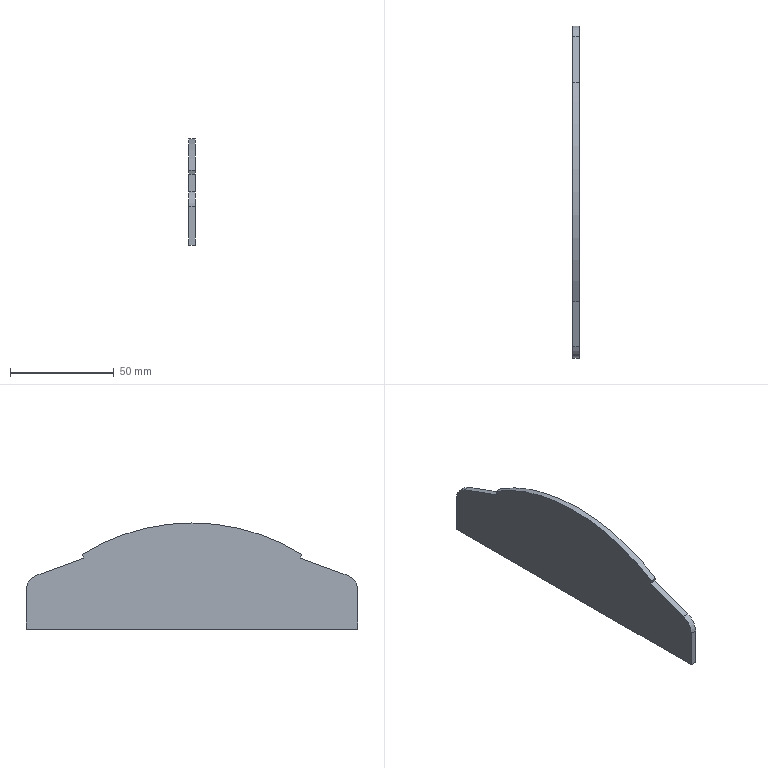Part | STEP file | 1-43.9 | 1 solid | 12 faces | box 3 x 160 x 51.122 mm | volume 19342 mm3 | plane 9 | cylinder 3 | commonest cylinder face diameters 16 x2 200 x1
STEP:
#1=CARTESIAN_POINT('',(0.,0.,0.));
#2=DIRECTION('',(0.,0.,1.));
#3=DIRECTION('',(1.,0.,0.));
#4=AXIS2_PLACEMENT_3D('',#1,#2,#3);
#5=CARTESIAN_POINT('',(0.,-80.,-12.));
#6=VERTEX_POINT('',#5);
#7=CARTESIAN_POINT('',(0.,80.,-12.));
#8=VERTEX_POINT('',#7);
#9=CARTESIAN_POINT('',(0.,-80.,-12.));
#10=DIRECTION('',(0.,1.,0.));
#11=VECTOR('',#10,1.);
#12=LINE('',#9,#11);
#13=CARTESIAN_POINT('',(0.,0.,68.));
#14=DIRECTION('',(1.,0.,0.));
#15=DIRECTION('',(0.,1.,0.));
#16=AXIS2_PLACEMENT_3D('',#13,#14,#15);
#17=PLANE('',#16);
#18=CARTESIAN_POINT('',(-80.,-80.));
#19=DIRECTION('',(1.,0.));
#20=VECTOR('',#19,1.);
#21=LINE('',#18,#20);
#22=(GEOMETRIC_REPRESENTATION_CONTEXT(2)PARAMETRIC_REPRESENTATION_CONTEXT()REPRESENTATION_CONTEXT('',''));
#23=DEFINITIONAL_REPRESENTATION('',(#21),#22);
#24=PCURVE('',#17,#23);
#25=CARTESIAN_POINT('',(-1.5,0.,-12.));
#26=DIRECTION('',(0.,0.,1.));
#27=DIRECTION('',(0.,1.,0.));
#28=AXIS2_PLACEMENT_3D('',#25,#26,#27);
#29=PLANE('',#28);
#30=CARTESIAN_POINT('',(-80.,-1.5));
#31=DIRECTION('',(1.,0.));
#32=VECTOR('',#31,1.);
#33=LINE('',#30,#32);
#34=(GEOMETRIC_REPRESENTATION_CONTEXT(2)PARAMETRIC_REPRESENTATION_CONTEXT()REPRESENTATION_CONTEXT('',''));
#35=DEFINITIONAL_REPRESENTATION('',(#33),#34);
#36=PCURVE('',#29,#35);
#37=SURFACE_CURVE('',#12,(#24,#36),.PCURVE_S1.);
#38=EDGE_CURVE('',#6,#8,#37,.T.);
#39=ORIENTED_EDGE('',*,*,#38,.T.);
#40=CARTESIAN_POINT('',(0.,80.,6.398));
#41=VERTEX_POINT('',#40);
#42=CARTESIAN_POINT('',(0.,80.,-12.));
#43=DIRECTION('',(0.,0.,1.));
#44=VECTOR('',#43,1.);
#45=LINE('',#42,#44);
#46=CARTESIAN_POINT('',(80.,-80.));
#47=DIRECTION('',(0.,1.));
#48=VECTOR('',#47,1.);
#49=LINE('',#46,#48);
#50=(GEOMETRIC_REPRESENTATION_CONTEXT(2)PARAMETRIC_REPRESENTATION_CONTEXT()REPRESENTATION_CONTEXT('',''));
#51=DEFINITIONAL_REPRESENTATION('',(#49),#50);
#52=PCURVE('',#17,#51);
#53=CARTESIAN_POINT('',(-1.5,80.,-2.801));
#54=DIRECTION('',(0.,-1.,0.));
#55=DIRECTION('',(0.,0.,1.));
#56=AXIS2_PLACEMENT_3D('',#53,#54,#55);
#57=PLANE('',#56);
#58=CARTESIAN_POINT('',(-9.199,-1.5));
#59=DIRECTION('',(1.,0.));
#60=VECTOR('',#59,1.);
#61=LINE('',#58,#60);
#62=(GEOMETRIC_REPRESENTATION_CONTEXT(2)PARAMETRIC_REPRESENTATION_CONTEXT()REPRESENTATION_CONTEXT('',''));
#63=DEFINITIONAL_REPRESENTATION('',(#61),#62);
#64=PCURVE('',#57,#63);
#65=SURFACE_CURVE('',#45,(#52,#64),.PCURVE_S1.);
#66=EDGE_CURVE('',#8,#41,#65,.T.);
#67=ORIENTED_EDGE('',*,*,#66,.T.);
#68=CARTESIAN_POINT('',(0.,74.736,13.916));
#69=VERTEX_POINT('',#68);
#70=CARTESIAN_POINT('',(0.,72.,6.398));
#71=DIRECTION('',(1.,0.,0.));
#72=DIRECTION('',(0.,1.,0.));
#73=AXIS2_PLACEMENT_3D('',#70,#71,#72);
#74=CIRCLE('',#73,8.);
#75=CARTESIAN_POINT('',(72.,-61.602));
#76=DIRECTION('',(1.,0.));
#77=AXIS2_PLACEMENT_2D('',#75,#76);
#78=CIRCLE('',#77,8.);
#79=(GEOMETRIC_REPRESENTATION_CONTEXT(2)PARAMETRIC_REPRESENTATION_CONTEXT()REPRESENTATION_CONTEXT('',''));
#80=DEFINITIONAL_REPRESENTATION('',(#78),#79);
#81=PCURVE('',#17,#80);
#82=CARTESIAN_POINT('',(0.,72.,6.398));
#83=DIRECTION('',(-1.,0.,0.));
#84=DIRECTION('',(0.,1.,0.));
#85=AXIS2_PLACEMENT_3D('',#82,#83,#84);
#86=CYLINDRICAL_SURFACE('',#85,8.);
#87=CARTESIAN_POINT('',(6.283,0.));
#88=DIRECTION('',(-1.,0.));
#89=VECTOR('',#88,1.);
#90=LINE('',#87,#89);
#91=(GEOMETRIC_REPRESENTATION_CONTEXT(2)PARAMETRIC_REPRESENTATION_CONTEXT()REPRESENTATION_CONTEXT('',''));
#92=DEFINITIONAL_REPRESENTATION('',(#90),#91);
#93=PCURVE('',#86,#92);
#94=SURFACE_CURVE('',#74,(#81,#93),.PCURVE_S1.);
#95=EDGE_CURVE('',#41,#69,#94,.T.);
#96=ORIENTED_EDGE('',*,*,#95,.T.);
#97=CARTESIAN_POINT('',(0.,52.185,22.124));
#98=VERTEX_POINT('',#97);
#99=CARTESIAN_POINT('',(0.,74.736,13.916));
#100=DIRECTION('',(0.,-0.9397,0.342));
#101=VECTOR('',#100,1.);
#102=LINE('',#99,#101);
#103=CARTESIAN_POINT('',(74.736,-54.084));
#104=DIRECTION('',(-0.9397,0.342));
#105=VECTOR('',#104,1.);
#106=LINE('',#103,#105);
#107=(GEOMETRIC_REPRESENTATION_CONTEXT(2)PARAMETRIC_REPRESENTATION_CONTEXT()REPRESENTATION_CONTEXT('',''));
#108=DEFINITIONAL_REPRESENTATION('',(#106),#107);
#109=PCURVE('',#17,#108);
#110=CARTESIAN_POINT('',(-1.5,63.461,18.02));
#111=DIRECTION('',(0.,-0.342,-0.9397));
#112=DIRECTION('',(0.,-0.9397,0.342));
#113=AXIS2_PLACEMENT_3D('',#110,#111,#112);
#114=PLANE('',#113);
#115=CARTESIAN_POINT('',(-11.999,-1.5));
#116=DIRECTION('',(1.,0.));
#117=VECTOR('',#116,1.);
#118=LINE('',#115,#117);
#119=(GEOMETRIC_REPRESENTATION_CONTEXT(2)PARAMETRIC_REPRESENTATION_CONTEXT()REPRESENTATION_CONTEXT('',''));
#120=DEFINITIONAL_REPRESENTATION('',(#118),#119);
#121=PCURVE('',#114,#120);
#122=SURFACE_CURVE('',#102,(#109,#121),.PCURVE_S1.);
#123=EDGE_CURVE('',#69,#98,#122,.T.);
#124=ORIENTED_EDGE('',*,*,#123,.T.);
#125=CARTESIAN_POINT('',(0.,52.869,24.003));
#126=VERTEX_POINT('',#125);
#127=CARTESIAN_POINT('',(0.,52.185,22.124));
#128=DIRECTION('',(0.,0.342,0.9397));
#129=VECTOR('',#128,1.);
#130=LINE('',#127,#129);
#131=CARTESIAN_POINT('',(52.185,-45.876));
#132=DIRECTION('',(0.342,0.9397));
#133=VECTOR('',#132,1.);
#134=LINE('',#131,#133);
#135=(GEOMETRIC_REPRESENTATION_CONTEXT(2)PARAMETRIC_REPRESENTATION_CONTEXT()REPRESENTATION_CONTEXT('',''));
#136=DEFINITIONAL_REPRESENTATION('',(#134),#135);
#137=PCURVE('',#17,#136);
#138=CARTESIAN_POINT('',(-1.5,52.527,23.063));
#139=DIRECTION('',(0.,-0.9397,0.342));
#140=DIRECTION('',(0.,0.342,0.9397));
#141=AXIS2_PLACEMENT_3D('',#138,#139,#140);
#142=PLANE('',#141);
#143=CARTESIAN_POINT('',(-1.,-1.5));
#144=DIRECTION('',(1.,0.));
#145=VECTOR('',#144,1.);
#146=LINE('',#143,#145);
#147=(GEOMETRIC_REPRESENTATION_CONTEXT(2)PARAMETRIC_REPRESENTATION_CONTEXT()REPRESENTATION_CONTEXT('',''));
#148=DEFINITIONAL_REPRESENTATION('',(#146),#147);
#149=PCURVE('',#142,#148);
#150=SURFACE_CURVE('',#130,(#137,#149),.PCURVE_S1.);
#151=EDGE_CURVE('',#98,#126,#150,.T.);
#152=ORIENTED_EDGE('',*,*,#151,.T.);
#153=CARTESIAN_POINT('',(0.,-52.869,24.003));
#154=VERTEX_POINT('',#153);
#155=CARTESIAN_POINT('',(0.,0.,-60.878));
#156=DIRECTION('',(1.,0.,0.));
#157=DIRECTION('',(0.,0.5287,0.8488));
#158=AXIS2_PLACEMENT_3D('',#155,#156,#157);
#159=CIRCLE('',#158,100.);
#160=CARTESIAN_POINT('',(0.,-128.878));
#161=DIRECTION('',(0.5287,0.8488));
#162=AXIS2_PLACEMENT_2D('',#160,#161);
#163=CIRCLE('',#162,100.);
#164=(GEOMETRIC_REPRESENTATION_CONTEXT(2)PARAMETRIC_REPRESENTATION_CONTEXT()REPRESENTATION_CONTEXT('',''));
#165=DEFINITIONAL_REPRESENTATION('',(#163),#164);
#166=PCURVE('',#17,#165);
#167=CARTESIAN_POINT('',(0.,0.,-60.878));
#168=DIRECTION('',(-1.,0.,0.));
#169=DIRECTION('',(0.,0.5287,0.8488));
#170=AXIS2_PLACEMENT_3D('',#167,#168,#169);
#171=CYLINDRICAL_SURFACE('',#170,100.);
#172=CARTESIAN_POINT('',(6.283,0.));
#173=DIRECTION('',(-1.,0.));
#174=VECTOR('',#173,1.);
#175=LINE('',#172,#174);
#176=(GEOMETRIC_REPRESENTATION_CONTEXT(2)PARAMETRIC_REPRESENTATION_CONTEXT()REPRESENTATION_CONTEXT('',''));
#177=DEFINITIONAL_REPRESENTATION('',(#175),#176);
#178=PCURVE('',#171,#177);
#179=SURFACE_CURVE('',#159,(#166,#178),.PCURVE_S1.);
#180=EDGE_CURVE('',#126,#154,#179,.T.);
#181=ORIENTED_EDGE('',*,*,#180,.T.);
#182=CARTESIAN_POINT('',(0.,-52.185,22.124));
#183=VERTEX_POINT('',#182);
#184=CARTESIAN_POINT('',(0.,-52.869,24.003));
#185=DIRECTION('',(0.,0.342,-0.9397));
#186=VECTOR('',#185,1.);
#187=LINE('',#184,#186);
#188=CARTESIAN_POINT('',(-52.869,-43.997));
#189=DIRECTION('',(0.342,-0.9397));
#190=VECTOR('',#189,1.);
#191=LINE('',#188,#190);
#192=(GEOMETRIC_REPRESENTATION_CONTEXT(2)PARAMETRIC_REPRESENTATION_CONTEXT()REPRESENTATION_CONTEXT('',''));
#193=DEFINITIONAL_REPRESENTATION('',(#191),#192);
#194=PCURVE('',#17,#193);
#195=CARTESIAN_POINT('',(-1.5,-52.527,23.063));
#196=DIRECTION('',(0.,0.9397,0.342));
#197=DIRECTION('',(0.,0.342,-0.9397));
#198=AXIS2_PLACEMENT_3D('',#195,#196,#197);
#199=PLANE('',#198);
#200=CARTESIAN_POINT('',(-1.,-1.5));
#201=DIRECTION('',(1.,0.));
#202=VECTOR('',#201,1.);
#203=LINE('',#200,#202);
#204=(GEOMETRIC_REPRESENTATION_CONTEXT(2)PARAMETRIC_REPRESENTATION_CONTEXT()REPRESENTATION_CONTEXT('',''));
#205=DEFINITIONAL_REPRESENTATION('',(#203),#204);
#206=PCURVE('',#199,#205);
#207=SURFACE_CURVE('',#187,(#194,#206),.PCURVE_S1.);
#208=EDGE_CURVE('',#154,#183,#207,.T.);
#209=ORIENTED_EDGE('',*,*,#208,.T.);
#210=CARTESIAN_POINT('',(0.,-74.736,13.916));
#211=VERTEX_POINT('',#210);
#212=CARTESIAN_POINT('',(0.,-52.185,22.124));
#213=DIRECTION('',(0.,-0.9397,-0.342));
#214=VECTOR('',#213,1.);
#215=LINE('',#212,#214);
#216=CARTESIAN_POINT('',(-52.185,-45.876));
#217=DIRECTION('',(-0.9397,-0.342));
#218=VECTOR('',#217,1.);
#219=LINE('',#216,#218);
#220=(GEOMETRIC_REPRESENTATION_CONTEXT(2)PARAMETRIC_REPRESENTATION_CONTEXT()REPRESENTATION_CONTEXT('',''));
#221=DEFINITIONAL_REPRESENTATION('',(#219),#220);
#222=PCURVE('',#17,#221);
#223=CARTESIAN_POINT('',(-1.5,-63.461,18.02));
#224=DIRECTION('',(0.,0.342,-0.9397));
#225=DIRECTION('',(0.,-0.9397,-0.342));
#226=AXIS2_PLACEMENT_3D('',#223,#224,#225);
#227=PLANE('',#226);
#228=CARTESIAN_POINT('',(-11.999,-1.5));
#229=DIRECTION('',(1.,0.));
#230=VECTOR('',#229,1.);
#231=LINE('',#228,#230);
#232=(GEOMETRIC_REPRESENTATION_CONTEXT(2)PARAMETRIC_REPRESENTATION_CONTEXT()REPRESENTATION_CONTEXT('',''));
#233=DEFINITIONAL_REPRESENTATION('',(#231),#232);
#234=PCURVE('',#227,#233);
#235=SURFACE_CURVE('',#215,(#222,#234),.PCURVE_S1.);
#236=EDGE_CURVE('',#183,#211,#235,.T.);
#237=ORIENTED_EDGE('',*,*,#236,.T.);
#238=CARTESIAN_POINT('',(0.,-80.,6.398));
#239=VERTEX_POINT('',#238);
#240=CARTESIAN_POINT('',(0.,-72.,6.398));
#241=DIRECTION('',(1.,0.,0.));
#242=DIRECTION('',(0.,-0.342,0.9397));
#243=AXIS2_PLACEMENT_3D('',#240,#241,#242);
#244=CIRCLE('',#243,8.);
#245=CARTESIAN_POINT('',(-72.,-61.602));
#246=DIRECTION('',(-0.342,0.9397));
#247=AXIS2_PLACEMENT_2D('',#245,#246);
#248=CIRCLE('',#247,8.);
#249=(GEOMETRIC_REPRESENTATION_CONTEXT(2)PARAMETRIC_REPRESENTATION_CONTEXT()REPRESENTATION_CONTEXT('',''));
#250=DEFINITIONAL_REPRESENTATION('',(#248),#249);
#251=PCURVE('',#17,#250);
#252=CARTESIAN_POINT('',(0.,-72.,6.398));
#253=DIRECTION('',(-1.,0.,0.));
#254=DIRECTION('',(0.,-0.342,0.9397));
#255=AXIS2_PLACEMENT_3D('',#252,#253,#254);
#256=CYLINDRICAL_SURFACE('',#255,8.);
#257=CARTESIAN_POINT('',(6.283,0.));
#258=DIRECTION('',(-1.,0.));
#259=VECTOR('',#258,1.);
#260=LINE('',#257,#259);
#261=(GEOMETRIC_REPRESENTATION_CONTEXT(2)PARAMETRIC_REPRESENTATION_CONTEXT()REPRESENTATION_CONTEXT('',''));
#262=DEFINITIONAL_REPRESENTATION('',(#260),#261);
#263=PCURVE('',#256,#262);
#264=SURFACE_CURVE('',#244,(#251,#263),.PCURVE_S1.);
#265=EDGE_CURVE('',#211,#239,#264,.T.);
#266=ORIENTED_EDGE('',*,*,#265,.T.);
#267=CARTESIAN_POINT('',(0.,-80.,6.398));
#268=DIRECTION('',(0.,0.,-1.));
#269=VECTOR('',#268,1.);
#270=LINE('',#267,#269);
#271=CARTESIAN_POINT('',(-80.,-61.602));
#272=DIRECTION('',(0.,-1.));
#273=VECTOR('',#272,1.);
#274=LINE('',#271,#273);
#275=(GEOMETRIC_REPRESENTATION_CONTEXT(2)PARAMETRIC_REPRESENTATION_CONTEXT()REPRESENTATION_CONTEXT('',''));
#276=DEFINITIONAL_REPRESENTATION('',(#274),#275);
#277=PCURVE('',#17,#276);
#278=CARTESIAN_POINT('',(-1.5,-80.,-2.801));
#279=DIRECTION('',(0.,1.,0.));
#280=DIRECTION('',(0.,0.,-1.));
#281=AXIS2_PLACEMENT_3D('',#278,#279,#280);
#282=PLANE('',#281);
#283=CARTESIAN_POINT('',(-9.199,-1.5));
#284=DIRECTION('',(1.,0.));
#285=VECTOR('',#284,1.);
#286=LINE('',#283,#285);
#287=(GEOMETRIC_REPRESENTATION_CONTEXT(2)PARAMETRIC_REPRESENTATION_CONTEXT()REPRESENTATION_CONTEXT('',''));
#288=DEFINITIONAL_REPRESENTATION('',(#286),#287);
#289=PCURVE('',#282,#288);
#290=SURFACE_CURVE('',#270,(#277,#289),.PCURVE_S1.);
#291=EDGE_CURVE('',#239,#6,#290,.T.);
#292=ORIENTED_EDGE('',*,*,#291,.T.);
#293=EDGE_LOOP('',(#39,#67,#96,#124,#152,#181,#209,#237,#266,#292));
#294=FACE_BOUND('',#293,.T.);
#295=ADVANCED_FACE('',(#294),#17,.T.);
#296=CARTESIAN_POINT('',(-3.,-80.,-12.));
#297=VERTEX_POINT('',#296);
#298=CARTESIAN_POINT('',(-3.,80.,-12.));
#299=VERTEX_POINT('',#298);
#300=CARTESIAN_POINT('',(-3.,-80.,-12.));
#301=DIRECTION('',(0.,1.,0.));
#302=VECTOR('',#301,1.);
#303=LINE('',#300,#302);
#304=CARTESIAN_POINT('',(-3.,0.,68.));
#305=DIRECTION('',(1.,0.,0.));
#306=DIRECTION('',(0.,1.,0.));
#307=AXIS2_PLACEMENT_3D('',#304,#305,#306);
#308=PLANE('',#307);
#309=CARTESIAN_POINT('',(-80.,-80.));
#310=DIRECTION('',(1.,0.));
#311=VECTOR('',#310,1.);
#312=LINE('',#309,#311);
#313=(GEOMETRIC_REPRESENTATION_CONTEXT(2)PARAMETRIC_REPRESENTATION_CONTEXT()REPRESENTATION_CONTEXT('',''));
#314=DEFINITIONAL_REPRESENTATION('',(#312),#313);
#315=PCURVE('',#308,#314);
#316=CARTESIAN_POINT('',(-80.,1.5));
#317=DIRECTION('',(1.,0.));
#318=VECTOR('',#317,1.);
#319=LINE('',#316,#318);
#320=(GEOMETRIC_REPRESENTATION_CONTEXT(2)PARAMETRIC_REPRESENTATION_CONTEXT()REPRESENTATION_CONTEXT('',''));
#321=DEFINITIONAL_REPRESENTATION('',(#319),#320);
#322=PCURVE('',#29,#321);
#323=SURFACE_CURVE('',#303,(#315,#322),.PCURVE_S1.);
#324=EDGE_CURVE('',#297,#299,#323,.T.);
#325=ORIENTED_EDGE('',*,*,#324,.T.);
#326=CARTESIAN_POINT('',(-3.,80.,6.398));
#327=VERTEX_POINT('',#326);
#328=CARTESIAN_POINT('',(-3.,80.,-12.));
#329=DIRECTION('',(0.,0.,1.));
#330=VECTOR('',#329,1.);
#331=LINE('',#328,#330);
#332=CARTESIAN_POINT('',(80.,-80.));
#333=DIRECTION('',(0.,1.));
#334=VECTOR('',#333,1.);
#335=LINE('',#332,#334);
#336=(GEOMETRIC_REPRESENTATION_CONTEXT(2)PARAMETRIC_REPRESENTATION_CONTEXT()REPRESENTATION_CONTEXT('',''));
#337=DEFINITIONAL_REPRESENTATION('',(#335),#336);
#338=PCURVE('',#308,#337);
#339=CARTESIAN_POINT('',(-9.199,1.5));
#340=DIRECTION('',(1.,0.));
#341=VECTOR('',#340,1.);
#342=LINE('',#339,#341);
#343=(GEOMETRIC_REPRESENTATION_CONTEXT(2)PARAMETRIC_REPRESENTATION_CONTEXT()REPRESENTATION_CONTEXT('',''));
#344=DEFINITIONAL_REPRESENTATION('',(#342),#343);
#345=PCURVE('',#57,#344);
#346=SURFACE_CURVE('',#331,(#338,#345),.PCURVE_S1.);
#347=EDGE_CURVE('',#299,#327,#346,.T.);
#348=ORIENTED_EDGE('',*,*,#347,.T.);
#349=CARTESIAN_POINT('',(-3.,74.736,13.916));
#350=VERTEX_POINT('',#349);
#351=CARTESIAN_POINT('',(-3.,72.,6.398));
#352=DIRECTION('',(1.,0.,0.));
#353=DIRECTION('',(0.,1.,0.));
#354=AXIS2_PLACEMENT_3D('',#351,#352,#353);
#355=CIRCLE('',#354,8.);
#356=CARTESIAN_POINT('',(72.,-61.602));
#357=DIRECTION('',(1.,0.));
#358=AXIS2_PLACEMENT_2D('',#356,#357);
#359=CIRCLE('',#358,8.);
#360=(GEOMETRIC_REPRESENTATION_CONTEXT(2)PARAMETRIC_REPRESENTATION_CONTEXT()REPRESENTATION_CONTEXT('',''));
#361=DEFINITIONAL_REPRESENTATION('',(#359),#360);
#362=PCURVE('',#308,#361);
#363=CARTESIAN_POINT('',(6.283,3.));
#364=DIRECTION('',(-1.,0.));
#365=VECTOR('',#364,1.);
#366=LINE('',#363,#365);
#367=(GEOMETRIC_REPRESENTATION_CONTEXT(2)PARAMETRIC_REPRESENTATION_CONTEXT()REPRESENTATION_CONTEXT('',''));
#368=DEFINITIONAL_REPRESENTATION('',(#366),#367);
#369=PCURVE('',#86,#368);
#370=SURFACE_CURVE('',#355,(#362,#369),.PCURVE_S1.);
#371=EDGE_CURVE('',#327,#350,#370,.T.);
#372=ORIENTED_EDGE('',*,*,#371,.T.);
#373=CARTESIAN_POINT('',(-3.,52.185,22.124));
#374=VERTEX_POINT('',#373);
#375=CARTESIAN_POINT('',(-3.,74.736,13.916));
#376=DIRECTION('',(0.,-0.9397,0.342));
#377=VECTOR('',#376,1.);
#378=LINE('',#375,#377);
#379=CARTESIAN_POINT('',(74.736,-54.084));
#380=DIRECTION('',(-0.9397,0.342));
#381=VECTOR('',#380,1.);
#382=LINE('',#379,#381);
#383=(GEOMETRIC_REPRESENTATION_CONTEXT(2)PARAMETRIC_REPRESENTATION_CONTEXT()REPRESENTATION_CONTEXT('',''));
#384=DEFINITIONAL_REPRESENTATION('',(#382),#383);
#385=PCURVE('',#308,#384);
#386=CARTESIAN_POINT('',(-11.999,1.5));
#387=DIRECTION('',(1.,0.));
#388=VECTOR('',#387,1.);
#389=LINE('',#386,#388);
#390=(GEOMETRIC_REPRESENTATION_CONTEXT(2)PARAMETRIC_REPRESENTATION_CONTEXT()REPRESENTATION_CONTEXT('',''));
#391=DEFINITIONAL_REPRESENTATION('',(#389),#390);
#392=PCURVE('',#114,#391);
#393=SURFACE_CURVE('',#378,(#385,#392),.PCURVE_S1.);
#394=EDGE_CURVE('',#350,#374,#393,.T.);
#395=ORIENTED_EDGE('',*,*,#394,.T.);
#396=CARTESIAN_POINT('',(-3.,52.869,24.003));
#397=VERTEX_POINT('',#396);
#398=CARTESIAN_POINT('',(-3.,52.185,22.124));
#399=DIRECTION('',(0.,0.342,0.9397));
#400=VECTOR('',#399,1.);
#401=LINE('',#398,#400);
#402=CARTESIAN_POINT('',(52.185,-45.876));
#403=DIRECTION('',(0.342,0.9397));
#404=VECTOR('',#403,1.);
#405=LINE('',#402,#404);
#406=(GEOMETRIC_REPRESENTATION_CONTEXT(2)PARAMETRIC_REPRESENTATION_CONTEXT()REPRESENTATION_CONTEXT('',''));
#407=DEFINITIONAL_REPRESENTATION('',(#405),#406);
#408=PCURVE('',#308,#407);
#409=CARTESIAN_POINT('',(-1.,1.5));
#410=DIRECTION('',(1.,0.));
#411=VECTOR('',#410,1.);
#412=LINE('',#409,#411);
#413=(GEOMETRIC_REPRESENTATION_CONTEXT(2)PARAMETRIC_REPRESENTATION_CONTEXT()REPRESENTATION_CONTEXT('',''));
#414=DEFINITIONAL_REPRESENTATION('',(#412),#413);
#415=PCURVE('',#142,#414);
#416=SURFACE_CURVE('',#401,(#408,#415),.PCURVE_S1.);
#417=EDGE_CURVE('',#374,#397,#416,.T.);
#418=ORIENTED_EDGE('',*,*,#417,.T.);
#419=CARTESIAN_POINT('',(-3.,-52.869,24.003));
#420=VERTEX_POINT('',#419);
#421=CARTESIAN_POINT('',(-3.,0.,-60.878));
#422=DIRECTION('',(1.,0.,0.));
#423=DIRECTION('',(0.,0.5287,0.8488));
#424=AXIS2_PLACEMENT_3D('',#421,#422,#423);
#425=CIRCLE('',#424,100.);
#426=CARTESIAN_POINT('',(0.,-128.878));
#427=DIRECTION('',(0.5287,0.8488));
#428=AXIS2_PLACEMENT_2D('',#426,#427);
#429=CIRCLE('',#428,100.);
#430=(GEOMETRIC_REPRESENTATION_CONTEXT(2)PARAMETRIC_REPRESENTATION_CONTEXT()REPRESENTATION_CONTEXT('',''));
#431=DEFINITIONAL_REPRESENTATION('',(#429),#430);
#432=PCURVE('',#308,#431);
#433=CARTESIAN_POINT('',(6.283,3.));
#434=DIRECTION('',(-1.,0.));
#435=VECTOR('',#434,1.);
#436=LINE('',#433,#435);
#437=(GEOMETRIC_REPRESENTATION_CONTEXT(2)PARAMETRIC_REPRESENTATION_CONTEXT()REPRESENTATION_CONTEXT('',''));
#438=DEFINITIONAL_REPRESENTATION('',(#436),#437);
#439=PCURVE('',#171,#438);
#440=SURFACE_CURVE('',#425,(#432,#439),.PCURVE_S1.);
#441=EDGE_CURVE('',#397,#420,#440,.T.);
#442=ORIENTED_EDGE('',*,*,#441,.T.);
#443=CARTESIAN_POINT('',(-3.,-52.185,22.124));
#444=VERTEX_POINT('',#443);
#445=CARTESIAN_POINT('',(-3.,-52.869,24.003));
#446=DIRECTION('',(0.,0.342,-0.9397));
#447=VECTOR('',#446,1.);
#448=LINE('',#445,#447);
#449=CARTESIAN_POINT('',(-52.869,-43.997));
#450=DIRECTION('',(0.342,-0.9397));
#451=VECTOR('',#450,1.);
#452=LINE('',#449,#451);
#453=(GEOMETRIC_REPRESENTATION_CONTEXT(2)PARAMETRIC_REPRESENTATION_CONTEXT()REPRESENTATION_CONTEXT('',''));
#454=DEFINITIONAL_REPRESENTATION('',(#452),#453);
#455=PCURVE('',#308,#454);
#456=CARTESIAN_POINT('',(-1.,1.5));
#457=DIRECTION('',(1.,0.));
#458=VECTOR('',#457,1.);
#459=LINE('',#456,#458);
#460=(GEOMETRIC_REPRESENTATION_CONTEXT(2)PARAMETRIC_REPRESENTATION_CONTEXT()REPRESENTATION_CONTEXT('',''));
#461=DEFINITIONAL_REPRESENTATION('',(#459),#460);
#462=PCURVE('',#199,#461);
#463=SURFACE_CURVE('',#448,(#455,#462),.PCURVE_S1.);
#464=EDGE_CURVE('',#420,#444,#463,.T.);
#465=ORIENTED_EDGE('',*,*,#464,.T.);
#466=CARTESIAN_POINT('',(-3.,-74.736,13.916));
#467=VERTEX_POINT('',#466);
#468=CARTESIAN_POINT('',(-3.,-52.185,22.124));
#469=DIRECTION('',(0.,-0.9397,-0.342));
#470=VECTOR('',#469,1.);
#471=LINE('',#468,#470);
#472=CARTESIAN_POINT('',(-52.185,-45.876));
#473=DIRECTION('',(-0.9397,-0.342));
#474=VECTOR('',#473,1.);
#475=LINE('',#472,#474);
#476=(GEOMETRIC_REPRESENTATION_CONTEXT(2)PARAMETRIC_REPRESENTATION_CONTEXT()REPRESENTATION_CONTEXT('',''));
#477=DEFINITIONAL_REPRESENTATION('',(#475),#476);
#478=PCURVE('',#308,#477);
#479=CARTESIAN_POINT('',(-11.999,1.5));
#480=DIRECTION('',(1.,0.));
#481=VECTOR('',#480,1.);
#482=LINE('',#479,#481);
#483=(GEOMETRIC_REPRESENTATION_CONTEXT(2)PARAMETRIC_REPRESENTATION_CONTEXT()REPRESENTATION_CONTEXT('',''));
#484=DEFINITIONAL_REPRESENTATION('',(#482),#483);
#485=PCURVE('',#227,#484);
#486=SURFACE_CURVE('',#471,(#478,#485),.PCURVE_S1.);
#487=EDGE_CURVE('',#444,#467,#486,.T.);
#488=ORIENTED_EDGE('',*,*,#487,.T.);
#489=CARTESIAN_POINT('',(-3.,-80.,6.398));
#490=VERTEX_POINT('',#489);
#491=CARTESIAN_POINT('',(-3.,-72.,6.398));
#492=DIRECTION('',(1.,0.,0.));
#493=DIRECTION('',(0.,-0.342,0.9397));
#494=AXIS2_PLACEMENT_3D('',#491,#492,#493);
#495=CIRCLE('',#494,8.);
#496=CARTESIAN_POINT('',(-72.,-61.602));
#497=DIRECTION('',(-0.342,0.9397));
#498=AXIS2_PLACEMENT_2D('',#496,#497);
#499=CIRCLE('',#498,8.);
#500=(GEOMETRIC_REPRESENTATION_CONTEXT(2)PARAMETRIC_REPRESENTATION_CONTEXT()REPRESENTATION_CONTEXT('',''));
#501=DEFINITIONAL_REPRESENTATION('',(#499),#500);
#502=PCURVE('',#308,#501);
#503=CARTESIAN_POINT('',(6.283,3.));
#504=DIRECTION('',(-1.,0.));
#505=VECTOR('',#504,1.);
#506=LINE('',#503,#505);
#507=(GEOMETRIC_REPRESENTATION_CONTEXT(2)PARAMETRIC_REPRESENTATION_CONTEXT()REPRESENTATION_CONTEXT('',''));
#508=DEFINITIONAL_REPRESENTATION('',(#506),#507);
#509=PCURVE('',#256,#508);
#510=SURFACE_CURVE('',#495,(#502,#509),.PCURVE_S1.);
#511=EDGE_CURVE('',#467,#490,#510,.T.);
#512=ORIENTED_EDGE('',*,*,#511,.T.);
#513=CARTESIAN_POINT('',(-3.,-80.,6.398));
#514=DIRECTION('',(0.,0.,-1.));
#515=VECTOR('',#514,1.);
#516=LINE('',#513,#515);
#517=CARTESIAN_POINT('',(-80.,-61.602));
#518=DIRECTION('',(0.,-1.));
#519=VECTOR('',#518,1.);
#520=LINE('',#517,#519);
#521=(GEOMETRIC_REPRESENTATION_CONTEXT(2)PARAMETRIC_REPRESENTATION_CONTEXT()REPRESENTATION_CONTEXT('',''));
#522=DEFINITIONAL_REPRESENTATION('',(#520),#521);
#523=PCURVE('',#308,#522);
#524=CARTESIAN_POINT('',(-9.199,1.5));
#525=DIRECTION('',(1.,0.));
#526=VECTOR('',#525,1.);
#527=LINE('',#524,#526);
#528=(GEOMETRIC_REPRESENTATION_CONTEXT(2)PARAMETRIC_REPRESENTATION_CONTEXT()REPRESENTATION_CONTEXT('',''));
#529=DEFINITIONAL_REPRESENTATION('',(#527),#528);
#530=PCURVE('',#282,#529);
#531=SURFACE_CURVE('',#516,(#523,#530),.PCURVE_S1.);
#532=EDGE_CURVE('',#490,#297,#531,.T.);
#533=ORIENTED_EDGE('',*,*,#532,.T.);
#534=EDGE_LOOP('',(#325,#348,#372,#395,#418,#442,#465,#488,#512,#533));
#535=FACE_BOUND('',#534,.F.);
#536=ADVANCED_FACE('',(#535),#308,.F.);
#537=ORIENTED_EDGE('',*,*,#38,.T.);
#538=CARTESIAN_POINT('',(0.,80.,-12.));
#539=DIRECTION('',(-1.,0.,0.));
#540=VECTOR('',#539,1.);
#541=LINE('',#538,#540);
#542=CARTESIAN_POINT('',(80.,-1.5));
#543=DIRECTION('',(0.,1.));
#544=VECTOR('',#543,1.);
#545=LINE('',#542,#544);
#546=(GEOMETRIC_REPRESENTATION_CONTEXT(2)PARAMETRIC_REPRESENTATION_CONTEXT()REPRESENTATION_CONTEXT('',''));
#547=DEFINITIONAL_REPRESENTATION('',(#545),#546);
#548=PCURVE('',#29,#547);
#549=CARTESIAN_POINT('',(-9.199,-1.5));
#550=DIRECTION('',(0.,1.));
#551=VECTOR('',#550,1.);
#552=LINE('',#549,#551);
#553=(GEOMETRIC_REPRESENTATION_CONTEXT(2)PARAMETRIC_REPRESENTATION_CONTEXT()REPRESENTATION_CONTEXT('',''));
#554=DEFINITIONAL_REPRESENTATION('',(#552),#553);
#555=PCURVE('',#57,#554);
#556=SURFACE_CURVE('',#541,(#548,#555),.PCURVE_S1.);
#557=EDGE_CURVE('',#8,#299,#556,.T.);
#558=ORIENTED_EDGE('',*,*,#557,.T.);
#559=ORIENTED_EDGE('',*,*,#324,.F.);
#560=CARTESIAN_POINT('',(0.,-80.,-12.));
#561=DIRECTION('',(-1.,0.,0.));
#562=VECTOR('',#561,1.);
#563=LINE('',#560,#562);
#564=CARTESIAN_POINT('',(-80.,-1.5));
#565=DIRECTION('',(0.,1.));
#566=VECTOR('',#565,1.);
#567=LINE('',#564,#566);
#568=(GEOMETRIC_REPRESENTATION_CONTEXT(2)PARAMETRIC_REPRESENTATION_CONTEXT()REPRESENTATION_CONTEXT('',''));
#569=DEFINITIONAL_REPRESENTATION('',(#567),#568);
#570=PCURVE('',#29,#569);
#571=CARTESIAN_POINT('',(9.199,-1.5));
#572=DIRECTION('',(0.,1.));
#573=VECTOR('',#572,1.);
#574=LINE('',#571,#573);
#575=(GEOMETRIC_REPRESENTATION_CONTEXT(2)PARAMETRIC_REPRESENTATION_CONTEXT()REPRESENTATION_CONTEXT('',''));
#576=DEFINITIONAL_REPRESENTATION('',(#574),#575);
#577=PCURVE('',#282,#576);
#578=SURFACE_CURVE('',#563,(#570,#577),.PCURVE_S1.);
#579=EDGE_CURVE('',#6,#297,#578,.T.);
#580=ORIENTED_EDGE('',*,*,#579,.F.);
#581=EDGE_LOOP('',(#537,#558,#559,#580));
#582=FACE_BOUND('',#581,.F.);
#583=ADVANCED_FACE('',(#582),#29,.F.);
#584=ORIENTED_EDGE('',*,*,#66,.T.);
#585=CARTESIAN_POINT('',(0.,80.,6.398));
#586=DIRECTION('',(-1.,0.,0.));
#587=VECTOR('',#586,1.);
#588=LINE('',#585,#587);
#589=CARTESIAN_POINT('',(9.199,-1.5));
#590=DIRECTION('',(0.,1.));
#591=VECTOR('',#590,1.);
#592=LINE('',#589,#591);
#593=(GEOMETRIC_REPRESENTATION_CONTEXT(2)PARAMETRIC_REPRESENTATION_CONTEXT()REPRESENTATION_CONTEXT('',''));
#594=DEFINITIONAL_REPRESENTATION('',(#592),#593);
#595=PCURVE('',#57,#594);
#596=CARTESIAN_POINT('',(6.283,0.));
#597=DIRECTION('',(0.,1.));
#598=VECTOR('',#597,1.);
#599=LINE('',#596,#598);
#600=(GEOMETRIC_REPRESENTATION_CONTEXT(2)PARAMETRIC_REPRESENTATION_CONTEXT()REPRESENTATION_CONTEXT('',''));
#601=DEFINITIONAL_REPRESENTATION('',(#599),#600);
#602=PCURVE('',#86,#601);
#603=SURFACE_CURVE('',#588,(#595,#602),.PCURVE_S1.);
#604=EDGE_CURVE('',#41,#327,#603,.T.);
#605=ORIENTED_EDGE('',*,*,#604,.T.);
#606=ORIENTED_EDGE('',*,*,#347,.F.);
#607=ORIENTED_EDGE('',*,*,#557,.F.);
#608=EDGE_LOOP('',(#584,#605,#606,#607));
#609=FACE_BOUND('',#608,.F.);
#610=ADVANCED_FACE('',(#609),#57,.F.);
#611=ORIENTED_EDGE('',*,*,#604,.T.);
#612=ORIENTED_EDGE('',*,*,#371,.T.);
#613=CARTESIAN_POINT('',(0.,74.736,13.916));
#614=DIRECTION('',(-1.,0.,0.));
#615=VECTOR('',#614,1.);
#616=LINE('',#613,#615);
#617=CARTESIAN_POINT('',(5.061,0.));
#618=DIRECTION('',(0.,1.));
#619=VECTOR('',#618,1.);
#620=LINE('',#617,#619);
#621=(GEOMETRIC_REPRESENTATION_CONTEXT(2)PARAMETRIC_REPRESENTATION_CONTEXT()REPRESENTATION_CONTEXT('',''));
#622=DEFINITIONAL_REPRESENTATION('',(#620),#621);
#623=PCURVE('',#86,#622);
#624=CARTESIAN_POINT('',(-11.999,-1.5));
#625=DIRECTION('',(0.,1.));
#626=VECTOR('',#625,1.);
#627=LINE('',#624,#626);
#628=(GEOMETRIC_REPRESENTATION_CONTEXT(2)PARAMETRIC_REPRESENTATION_CONTEXT()REPRESENTATION_CONTEXT('',''));
#629=DEFINITIONAL_REPRESENTATION('',(#627),#628);
#630=PCURVE('',#114,#629);
#631=SURFACE_CURVE('',#616,(#623,#630),.PCURVE_S1.);
#632=EDGE_CURVE('',#69,#350,#631,.T.);
#633=ORIENTED_EDGE('',*,*,#632,.F.);
#634=ORIENTED_EDGE('',*,*,#95,.F.);
#635=EDGE_LOOP('',(#611,#612,#633,#634));
#636=FACE_BOUND('',#635,.T.);
#637=ADVANCED_FACE('',(#636),#86,.T.);
#638=ORIENTED_EDGE('',*,*,#123,.T.);
#639=CARTESIAN_POINT('',(0.,52.185,22.124));
#640=DIRECTION('',(-1.,0.,0.));
#641=VECTOR('',#640,1.);
#642=LINE('',#639,#641);
#643=CARTESIAN_POINT('',(11.999,-1.5));
#644=DIRECTION('',(0.,1.));
#645=VECTOR('',#644,1.);
#646=LINE('',#643,#645);
#647=(GEOMETRIC_REPRESENTATION_CONTEXT(2)PARAMETRIC_REPRESENTATION_CONTEXT()REPRESENTATION_CONTEXT('',''));
#648=DEFINITIONAL_REPRESENTATION('',(#646),#647);
#649=PCURVE('',#114,#648);
#650=CARTESIAN_POINT('',(-1.,-1.5));
#651=DIRECTION('',(0.,1.));
#652=VECTOR('',#651,1.);
#653=LINE('',#650,#652);
#654=(GEOMETRIC_REPRESENTATION_CONTEXT(2)PARAMETRIC_REPRESENTATION_CONTEXT()REPRESENTATION_CONTEXT('',''));
#655=DEFINITIONAL_REPRESENTATION('',(#653),#654);
#656=PCURVE('',#142,#655);
#657=SURFACE_CURVE('',#642,(#649,#656),.PCURVE_S1.);
#658=EDGE_CURVE('',#98,#374,#657,.T.);
#659=ORIENTED_EDGE('',*,*,#658,.T.);
#660=ORIENTED_EDGE('',*,*,#394,.F.);
#661=ORIENTED_EDGE('',*,*,#632,.F.);
#662=EDGE_LOOP('',(#638,#659,#660,#661));
#663=FACE_BOUND('',#662,.F.);
#664=ADVANCED_FACE('',(#663),#114,.F.);
#665=ORIENTED_EDGE('',*,*,#151,.T.);
#666=CARTESIAN_POINT('',(0.,52.869,24.003));
#667=DIRECTION('',(-1.,0.,0.));
#668=VECTOR('',#667,1.);
#669=LINE('',#666,#668);
#670=CARTESIAN_POINT('',(1.,-1.5));
#671=DIRECTION('',(0.,1.));
#672=VECTOR('',#671,1.);
#673=LINE('',#670,#672);
#674=(GEOMETRIC_REPRESENTATION_CONTEXT(2)PARAMETRIC_REPRESENTATION_CONTEXT()REPRESENTATION_CONTEXT('',''));
#675=DEFINITIONAL_REPRESENTATION('',(#673),#674);
#676=PCURVE('',#142,#675);
#677=CARTESIAN_POINT('',(6.283,0.));
#678=DIRECTION('',(0.,1.));
#679=VECTOR('',#678,1.);
#680=LINE('',#677,#679);
#681=(GEOMETRIC_REPRESENTATION_CONTEXT(2)PARAMETRIC_REPRESENTATION_CONTEXT()REPRESENTATION_CONTEXT('',''));
#682=DEFINITIONAL_REPRESENTATION('',(#680),#681);
#683=PCURVE('',#171,#682);
#684=SURFACE_CURVE('',#669,(#676,#683),.PCURVE_S1.);
#685=EDGE_CURVE('',#126,#397,#684,.T.);
#686=ORIENTED_EDGE('',*,*,#685,.T.);
#687=ORIENTED_EDGE('',*,*,#417,.F.);
#688=ORIENTED_EDGE('',*,*,#658,.F.);
#689=EDGE_LOOP('',(#665,#686,#687,#688));
#690=FACE_BOUND('',#689,.F.);
#691=ADVANCED_FACE('',(#690),#142,.F.);
#692=ORIENTED_EDGE('',*,*,#685,.T.);
#693=ORIENTED_EDGE('',*,*,#441,.T.);
#694=CARTESIAN_POINT('',(0.,-52.869,24.003));
#695=DIRECTION('',(-1.,0.,0.));
#696=VECTOR('',#695,1.);
#697=LINE('',#694,#696);
#698=CARTESIAN_POINT('',(5.169,0.));
#699=DIRECTION('',(0.,1.));
#700=VECTOR('',#699,1.);
#701=LINE('',#698,#700);
#702=(GEOMETRIC_REPRESENTATION_CONTEXT(2)PARAMETRIC_REPRESENTATION_CONTEXT()REPRESENTATION_CONTEXT('',''));
#703=DEFINITIONAL_REPRESENTATION('',(#701),#702);
#704=PCURVE('',#171,#703);
#705=CARTESIAN_POINT('',(-1.,-1.5));
#706=DIRECTION('',(0.,1.));
#707=VECTOR('',#706,1.);
#708=LINE('',#705,#707);
#709=(GEOMETRIC_REPRESENTATION_CONTEXT(2)PARAMETRIC_REPRESENTATION_CONTEXT()REPRESENTATION_CONTEXT('',''));
#710=DEFINITIONAL_REPRESENTATION('',(#708),#709);
#711=PCURVE('',#199,#710);
#712=SURFACE_CURVE('',#697,(#704,#711),.PCURVE_S1.);
#713=EDGE_CURVE('',#154,#420,#712,.T.);
#714=ORIENTED_EDGE('',*,*,#713,.F.);
#715=ORIENTED_EDGE('',*,*,#180,.F.);
#716=EDGE_LOOP('',(#692,#693,#714,#715));
#717=FACE_BOUND('',#716,.T.);
#718=ADVANCED_FACE('',(#717),#171,.T.);
#719=ORIENTED_EDGE('',*,*,#208,.T.);
#720=CARTESIAN_POINT('',(0.,-52.185,22.124));
#721=DIRECTION('',(-1.,0.,0.));
#722=VECTOR('',#721,1.);
#723=LINE('',#720,#722);
#724=CARTESIAN_POINT('',(1.,-1.5));
#725=DIRECTION('',(0.,1.));
#726=VECTOR('',#725,1.);
#727=LINE('',#724,#726);
#728=(GEOMETRIC_REPRESENTATION_CONTEXT(2)PARAMETRIC_REPRESENTATION_CONTEXT()REPRESENTATION_CONTEXT('',''));
#729=DEFINITIONAL_REPRESENTATION('',(#727),#728);
#730=PCURVE('',#199,#729);
#731=CARTESIAN_POINT('',(-11.999,-1.5));
#732=DIRECTION('',(0.,1.));
#733=VECTOR('',#732,1.);
#734=LINE('',#731,#733);
#735=(GEOMETRIC_REPRESENTATION_CONTEXT(2)PARAMETRIC_REPRESENTATION_CONTEXT()REPRESENTATION_CONTEXT('',''));
#736=DEFINITIONAL_REPRESENTATION('',(#734),#735);
#737=PCURVE('',#227,#736);
#738=SURFACE_CURVE('',#723,(#730,#737),.PCURVE_S1.);
#739=EDGE_CURVE('',#183,#444,#738,.T.);
#740=ORIENTED_EDGE('',*,*,#739,.T.);
#741=ORIENTED_EDGE('',*,*,#464,.F.);
#742=ORIENTED_EDGE('',*,*,#713,.F.);
#743=EDGE_LOOP('',(#719,#740,#741,#742));
#744=FACE_BOUND('',#743,.F.);
#745=ADVANCED_FACE('',(#744),#199,.F.);
#746=ORIENTED_EDGE('',*,*,#236,.T.);
#747=CARTESIAN_POINT('',(0.,-74.736,13.916));
#748=DIRECTION('',(-1.,0.,0.));
#749=VECTOR('',#748,1.);
#750=LINE('',#747,#749);
#751=CARTESIAN_POINT('',(11.999,-1.5));
#752=DIRECTION('',(0.,1.));
#753=VECTOR('',#752,1.);
#754=LINE('',#751,#753);
#755=(GEOMETRIC_REPRESENTATION_CONTEXT(2)PARAMETRIC_REPRESENTATION_CONTEXT()REPRESENTATION_CONTEXT('',''));
#756=DEFINITIONAL_REPRESENTATION('',(#754),#755);
#757=PCURVE('',#227,#756);
#758=CARTESIAN_POINT('',(6.283,0.));
#759=DIRECTION('',(0.,1.));
#760=VECTOR('',#759,1.);
#761=LINE('',#758,#760);
#762=(GEOMETRIC_REPRESENTATION_CONTEXT(2)PARAMETRIC_REPRESENTATION_CONTEXT()REPRESENTATION_CONTEXT('',''));
#763=DEFINITIONAL_REPRESENTATION('',(#761),#762);
#764=PCURVE('',#256,#763);
#765=SURFACE_CURVE('',#750,(#757,#764),.PCURVE_S1.);
#766=EDGE_CURVE('',#211,#467,#765,.T.);
#767=ORIENTED_EDGE('',*,*,#766,.T.);
#768=ORIENTED_EDGE('',*,*,#487,.F.);
#769=ORIENTED_EDGE('',*,*,#739,.F.);
#770=EDGE_LOOP('',(#746,#767,#768,#769));
#771=FACE_BOUND('',#770,.F.);
#772=ADVANCED_FACE('',(#771),#227,.F.);
#773=ORIENTED_EDGE('',*,*,#766,.T.);
#774=ORIENTED_EDGE('',*,*,#511,.T.);
#775=CARTESIAN_POINT('',(0.,-80.,6.398));
#776=DIRECTION('',(-1.,0.,0.));
#777=VECTOR('',#776,1.);
#778=LINE('',#775,#777);
#779=CARTESIAN_POINT('',(5.061,0.));
#780=DIRECTION('',(0.,1.));
#781=VECTOR('',#780,1.);
#782=LINE('',#779,#781);
#783=(GEOMETRIC_REPRESENTATION_CONTEXT(2)PARAMETRIC_REPRESENTATION_CONTEXT()REPRESENTATION_CONTEXT('',''));
#784=DEFINITIONAL_REPRESENTATION('',(#782),#783);
#785=PCURVE('',#256,#784);
#786=CARTESIAN_POINT('',(-9.199,-1.5));
#787=DIRECTION('',(0.,1.));
#788=VECTOR('',#787,1.);
#789=LINE('',#786,#788);
#790=(GEOMETRIC_REPRESENTATION_CONTEXT(2)PARAMETRIC_REPRESENTATION_CONTEXT()REPRESENTATION_CONTEXT('',''));
#791=DEFINITIONAL_REPRESENTATION('',(#789),#790);
#792=PCURVE('',#282,#791);
#793=SURFACE_CURVE('',#778,(#785,#792),.PCURVE_S1.);
#794=EDGE_CURVE('',#239,#490,#793,.T.);
#795=ORIENTED_EDGE('',*,*,#794,.F.);
#796=ORIENTED_EDGE('',*,*,#265,.F.);
#797=EDGE_LOOP('',(#773,#774,#795,#796));
#798=FACE_BOUND('',#797,.T.);
#799=ADVANCED_FACE('',(#798),#256,.T.);
#800=ORIENTED_EDGE('',*,*,#291,.T.);
#801=ORIENTED_EDGE('',*,*,#579,.T.);
#802=ORIENTED_EDGE('',*,*,#532,.F.);
#803=ORIENTED_EDGE('',*,*,#794,.F.);
#804=EDGE_LOOP('',(#800,#801,#802,#803));
#805=FACE_BOUND('',#804,.F.);
#806=ADVANCED_FACE('',(#805),#282,.F.);
#807=CLOSED_SHELL('',(#295,#536,#583,#610,#637,#664,#691,#718,#745,#772,#799,#806));
#808=MANIFOLD_SOLID_BREP('',#807);
#809=(LENGTH_UNIT()NAMED_UNIT(*)SI_UNIT(.MILLI.,.METRE.));
#810=UNCERTAINTY_MEASURE_WITH_UNIT(LENGTH_MEASURE(0.0000001),#809,'','');
#811=(NAMED_UNIT(*)PLANE_ANGLE_UNIT()SI_UNIT($,.RADIAN.));
#812=(NAMED_UNIT(*)SI_UNIT($,.STERADIAN.)SOLID_ANGLE_UNIT());
#813=(GEOMETRIC_REPRESENTATION_CONTEXT(3)GLOBAL_UNCERTAINTY_ASSIGNED_CONTEXT((#810))GLOBAL_UNIT_ASSIGNED_CONTEXT((#809,#811,#812))REPRESENTATION_CONTEXT('',''));
#814=ADVANCED_BREP_SHAPE_REPRESENTATION('',(#4,#808),#813);